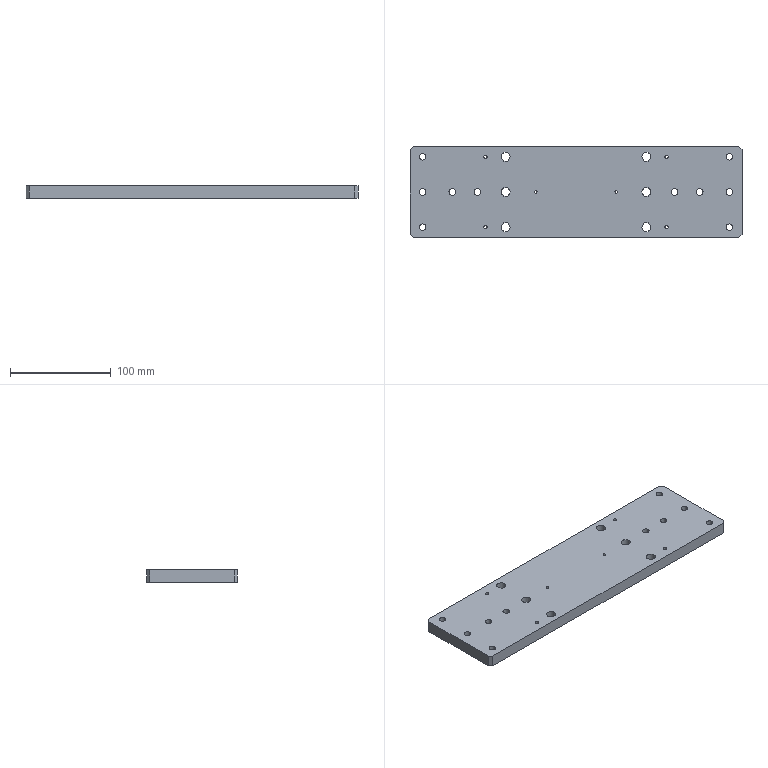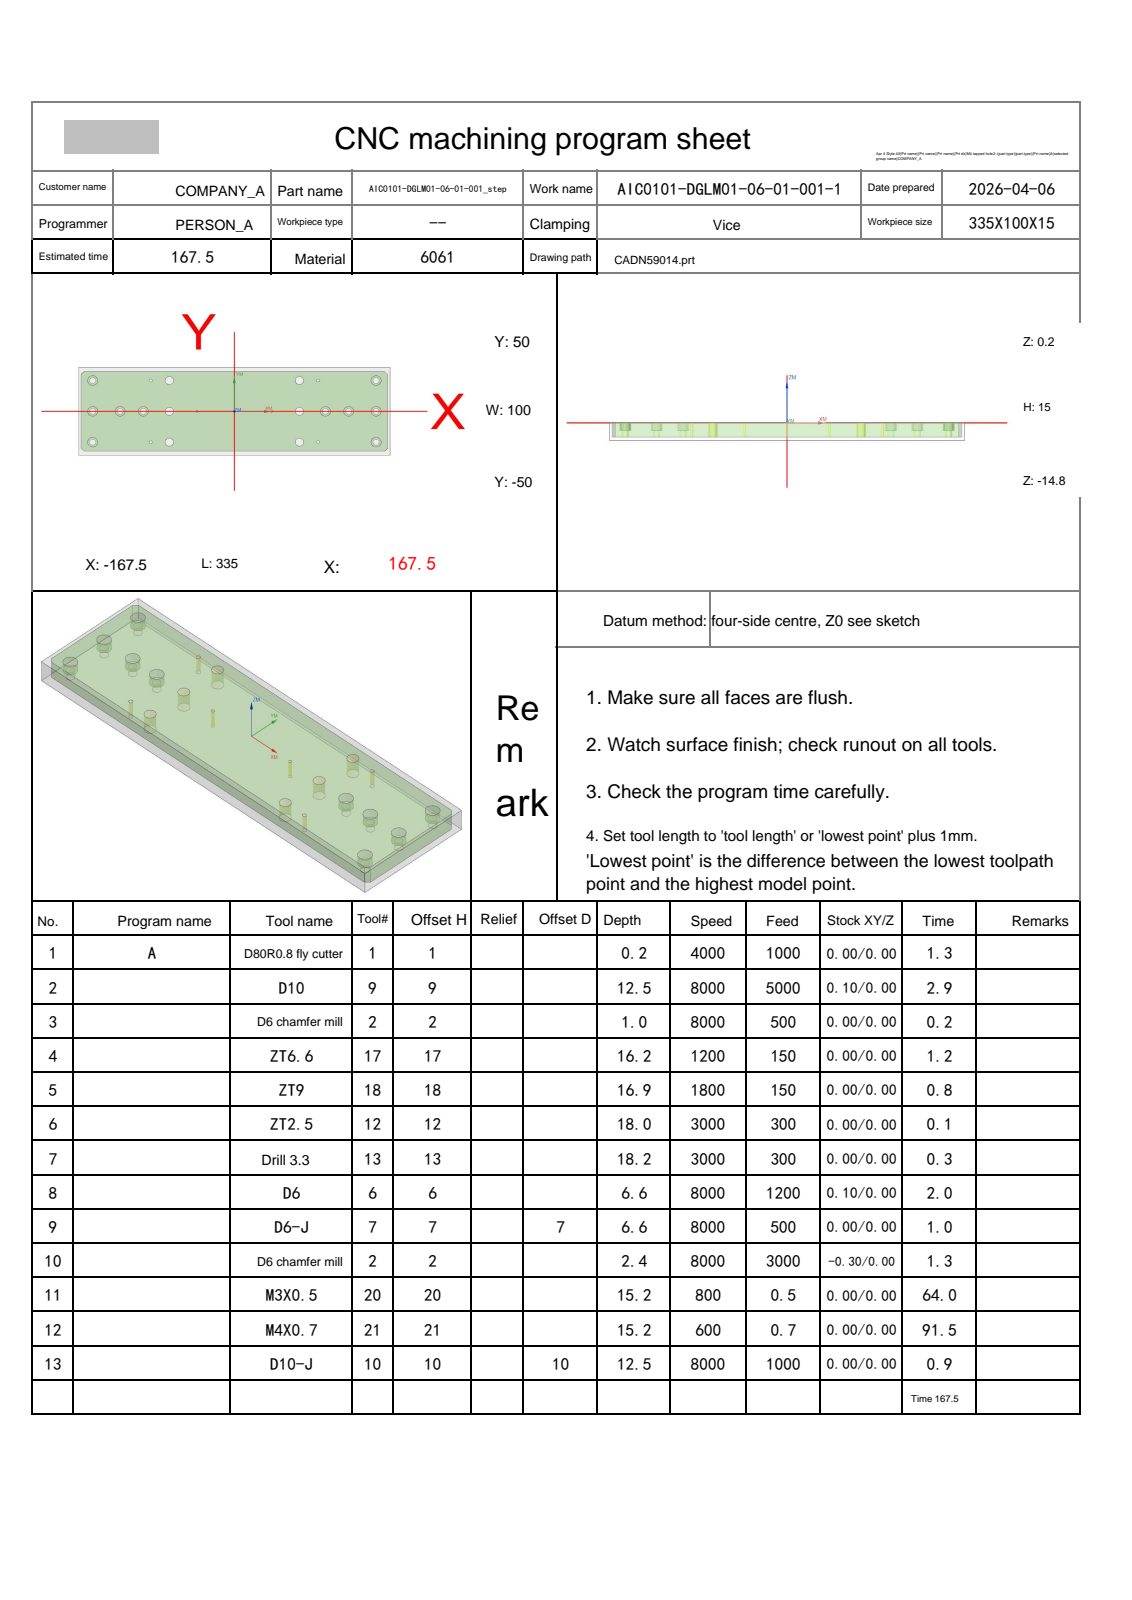NC program | NX | posted by the shop | part box 330 x 90 x 12 mm
Whole program:
%
O0001
(Machine time: 315.72 MIN)
(===Total Tool:12===)
(T1=D80R0.8 fly cutter D=80.  R=0.8  D-  H01 Z=0.    )
(T9=D10     D=10.  R=0.   D-  H09 Z=-12.3 )
(T2=D6 chamfer mill   D=6.   R=0.   D-  H02 Z=-2.2  )
(T17=ZT6.6  D=6.6  DR_a=118 D-  H17 Z=-15.98)
(T18=ZT9    D=9.   DR_a=118 D-  H18 Z=-16.7 )
(T12=ZT2.5  D=2.5  DR_a=118 D-  H12 Z=-17.75)
(T13=drill 3.3  D=3.3  DR_a=118 D-  H13 Z=-17.99)
(T6=D6      D=6.   R=0.   D-  H06 Z=-6.4  )
(T7=D6-J    D=6.   R=0.   D7  H07 Z=-6.4  )
(T20=M3X0.5 D=2.5  DR_a=180 D-  H20 Z=-15.  )
(T21=M4X0.7 D=3.3  DR_a=180 D-  H21 Z=-15.  )
(T10=D10-J  D=10.  R=0.   D10 H10 Z=-12.3 )
G80 G90 G17 G49 G40
G91 G28 Z0
M01
N1 T01 M06
(D80R0.8 fly cutter  D=80. R=0.8 H=01 ce=0.00 di=0.00)
G00 G90 G54 X210. Y-42.5 M03 S4000
G43 H01 Z20.
M08
Z2.
G01 Z0.0 F1000.
X205.
X-205.
Y0.0
X205.
Y42.5
X-205.
X-210.
Z2.
G00 Z20.
G91 G28 Z0.0
M05
M09
G91 G28 Z0.0
M01
N2 T09 M06
(D10  D=10. R=0. H=09 ce=0.10 di=0.00)
G00 G90 G54 X0.0 Y50.1 M03 S8000
G43 H09 Z20.
M08
Z.5
G01 X162. Z.35 F5000.
G02 X165.606 Y48.606 Z.346 I0.0 J-5.1
G01 X168.606 Y45.606 Z.343
G02 X170.1 Y42. Z.339 I-3.606 J-3.606
G01 Y-42. Z.261
G02 X168.606 Y-45.606 Z.257 I-5.1 J0.0
G01 X165.606 Y-48.606 Z.254
G02 X162. Y-50.1 Z.25 I-3.606 J3.606
G01 X-162. Z-.05
G02 X-165.606 Y-48.606 Z-.054 I0.0 J5.1
G01 X-168.606 Y-45.606 Z-.057
G02 X-170.1 Y-42. Z-.061 I3.606 J3.606
G01 Y42. Z-.139
G02 X-168.606 Y45.606 Z-.143 I5.1 J0.0
G01 X-165.606 Y48.606 Z-.146
G02 X-162. Y50.1 Z-.15 I3.606 J-3.606
G01 X162. Z-.45
G02 X165.606 Y48.606 Z-.454 I0.0 J-5.1
G01 X168.606 Y45.606 Z-.457
G02 X170.1 Y42. Z-.461 I-3.606 J-3.606
G01 Y-42. Z-.539
G02 X168.606 Y-45.606 Z-.543 I-5.1 J0.0
G01 X165.606 Y-48.606 Z-.546
G02 X162. Y-50.1 Z-.55 I-3.606 J3.606
G01 X-162. Z-.85
G02 X-165.606 Y-48.606 Z-.854 I0.0 J5.1
G01 X-168.606 Y-45.606 Z-.857
G02 X-170.1 Y-42. Z-.861 I3.606 J3.606
G01 Y42. Z-.939
G02 X-168.606 Y45.606 Z-.943 I5.1 J0.0
G01 X-165.606 Y48.606 Z-.946
G02 X-162. Y50.1 Z-.95 I3.606 J-3.606
G01 X162. Z-1.25
G02 X165.606 Y48.606 Z-1.254 I0.0 J-5.1
G01 X168.606 Y45.606 Z-1.257
G02 X170.1 Y42. Z-1.261 I-3.606 J-3.606
G01 Y-42. Z-1.339
G02 X168.606 Y-45.606 Z-1.343 I-5.1 J0.0
G01 X165.606 Y-48.606 Z-1.346
G02 X162. Y-50.1 Z-1.35 I-3.606 J3.606
G01 X-162. Z-1.65
G02 X-165.606 Y-48.606 Z-1.654 I0.0 J5.1
G01 X-168.606 Y-45.606 Z-1.657
G02 X-170.1 Y-42. Z-1.661 I3.606 J3.606
G01 Y42. Z-1.739
G02 X-168.606 Y45.606 Z-1.743 I5.1 J0.0
G01 X-165.606 Y48.606 Z-1.746
G02 X-162. Y50.1 Z-1.75 I3.606 J-3.606
G01 X162. Z-2.05
G02 X165.606 Y48.606 Z-2.054 I0.0 J-5.1
G01 X168.606 Y45.606 Z-2.057
G02 X170.1 Y42. Z-2.061 I-3.606 J-3.606
G01 Y-42. Z-2.139
G02 X168.606 Y-45.606 Z-2.143 I-5.1 J0.0
G01 X165.606 Y-48.606 Z-2.146
G02 X162. Y-50.1 Z-2.15 I-3.606 J3.606
G01 X-162. Z-2.45
G02 X-165.606 Y-48.606 Z-2.454 I0.0 J5.1
G01 X-168.606 Y-45.606 Z-2.457
G02 X-170.1 Y-42. Z-2.461 I3.606 J3.606
G01 Y42. Z-2.539
G02 X-168.606 Y45.606 Z-2.543 I5.1 J0.0
G01 X-165.606 Y48.606 Z-2.546
G02 X-162. Y50.1 Z-2.55 I3.606 J-3.606
G01 X162. Z-2.85
G02 X165.606 Y48.606 Z-2.854 I0.0 J-5.1
G01 X168.606 Y45.606 Z-2.857
G02 X170.1 Y42. Z-2.861 I-3.606 J-3.606
G01 Y-42. Z-2.939
G02 X168.606 Y-45.606 Z-2.943 I-5.1 J0.0
G01 X165.606 Y-48.606 Z-2.946
G02 X162. Y-50.1 Z-2.95 I-3.606 J3.606
G01 X-162. Z-3.25
G02 X-165.606 Y-48.606 Z-3.254 I0.0 J5.1
G01 X-168.606 Y-45.606 Z-3.257
G02 X-170.1 Y-42. Z-3.261 I3.606 J3.606
G01 Y42. Z-3.339
G02 X-168.606 Y45.606 Z-3.343 I5.1 J0.0
G01 X-165.606 Y48.606 Z-3.346
G02 X-162. Y50.1 Z-3.35 I3.606 J-3.606
G01 X162. Z-3.65
G02 X165.606 Y48.606 Z-3.654 I0.0 J-5.1
G01 X168.606 Y45.606 Z-3.657
G02 X170.1 Y42. Z-3.661 I-3.606 J-3.606
G01 Y-42. Z-3.739
G02 X168.606 Y-45.606 Z-3.743 I-5.1 J0.0
G01 X165.606 Y-48.606 Z-3.746
G02 X162. Y-50.1 Z-3.75 I-3.606 J3.606
G01 X-162. Z-4.05
G02 X-165.606 Y-48.606 Z-4.054 I0.0 J5.1
G01 X-168.606 Y-45.606 Z-4.057
G02 X-170.1 Y-42. Z-4.061 I3.606 J3.606
G01 Y42. Z-4.139
G02 X-168.606 Y45.606 Z-4.143 I5.1 J0.0
G01 X-165.606 Y48.606 Z-4.146
G02 X-162. Y50.1 Z-4.15 I3.606 J-3.606
G01 X162. Z-4.45
G02 X165.606 Y48.606 Z-4.454 I0.0 J-5.1
G01 X168.606 Y45.606 Z-4.457
G02 X170.1 Y42. Z-4.461 I-3.606 J-3.606
G01 Y-42. Z-4.539
G02 X168.606 Y-45.606 Z-4.543 I-5.1 J0.0
G01 X165.606 Y-48.606 Z-4.546
G02 X162. Y-50.1 Z-4.55 I-3.606 J3.606
G01 X-162. Z-4.85
G02 X-165.606 Y-48.606 Z-4.854 I0.0 J5.1
G01 X-168.606 Y-45.606 Z-4.857
G02 X-170.1 Y-42. Z-4.861 I3.606 J3.606
G01 Y42. Z-4.939
G02 X-168.606 Y45.606 Z-4.943 I5.1 J0.0
G01 X-165.606 Y48.606 Z-4.946
G02 X-162. Y50.1 Z-4.95 I3.606 J-3.606
G01 X162. Z-5.25
G02 X165.606 Y48.606 Z-5.254 I0.0 J-5.1
G01 X168.606 Y45.606 Z-5.257
G02 X170.1 Y42. Z-5.261 I-3.606 J-3.606
G01 Y-42. Z-5.339
G02 X168.606 Y-45.606 Z-5.343 I-5.1 J0.0
G01 X165.606 Y-48.606 Z-5.346
G02 X162. Y-50.1 Z-5.35 I-3.606 J3.606
G01 X-162. Z-5.65
G02 X-165.606 Y-48.606 Z-5.654 I0.0 J5.1
G01 X-168.606 Y-45.606 Z-5.657
G02 X-170.1 Y-42. Z-5.661 I3.606 J3.606
G01 Y42. Z-5.739
G02 X-168.606 Y45.606 Z-5.743 I5.1 J0.0
G01 X-165.606 Y48.606 Z-5.746
G02 X-162. Y50.1 Z-5.75 I3.606 J-3.606
G01 X162. Z-6.05
G02 X165.606 Y48.606 Z-6.054 I0.0 J-5.1
G01 X168.606 Y45.606 Z-6.057
G02 X170.1 Y42. Z-6.061 I-3.606 J-3.606
G01 Y-42. Z-6.139
G02 X168.606 Y-45.606 Z-6.143 I-5.1 J0.0
G01 X165.606 Y-48.606 Z-6.146
G02 X162. Y-50.1 Z-6.15 I-3.606 J3.606
G01 X-162. Z-6.45
G02 X-165.606 Y-48.606 Z-6.454 I0.0 J5.1
G01 X-168.606 Y-45.606 Z-6.457
G02 X-170.1 Y-42. Z-6.461 I3.606 J3.606
G01 Y42. Z-6.539
G02 X-168.606 Y45.606 Z-6.543 I5.1 J0.0
G01 X-165.606 Y48.606 Z-6.546
G02 X-162. Y50.1 Z-6.55 I3.606 J-3.606
G01 X162. Z-6.85
G02 X165.606 Y48.606 Z-6.854 I0.0 J-5.1
G01 X168.606 Y45.606 Z-6.857
G02 X170.1 Y42. Z-6.861 I-3.606 J-3.606
G01 Y-42. Z-6.939
G02 X168.606 Y-45.606 Z-6.943 I-5.1 J0.0
G01 X165.606 Y-48.606 Z-6.946
G02 X162. Y-50.1 Z-6.95 I-3.606 J3.606
G01 X-162. Z-7.25
G02 X-165.606 Y-48.606 Z-7.254 I0.0 J5.1
G01 X-168.606 Y-45.606 Z-7.257
G02 X-170.1 Y-42. Z-7.261 I3.606 J3.606
G01 Y42. Z-7.339
G02 X-168.606 Y45.606 Z-7.343 I5.1 J0.0
G01 X-165.606 Y48.606 Z-7.346
G02 X-162. Y50.1 Z-7.35 I3.606 J-3.606
G01 X162. Z-7.65
G02 X165.606 Y48.606 Z-7.654 I0.0 J-5.1
G01 X168.606 Y45.606 Z-7.657
G02 X170.1 Y42. Z-7.661 I-3.606 J-3.606
G01 Y-42. Z-7.739
G02 X168.606 Y-45.606 Z-7.743 I-5.1 J0.0
G01 X165.606 Y-48.606 Z-7.746
G02 X162. Y-50.1 Z-7.75 I-3.606 J3.606
G01 X-162. Z-8.05
G02 X-165.606 Y-48.606 Z-8.054 I0.0 J5.1
G01 X-168.606 Y-45.606 Z-8.057
G02 X-170.1 Y-42. Z-8.061 I3.606 J3.606
G01 Y42. Z-8.139
G02 X-168.606 Y45.606 Z-8.143 I5.1 J0.0
G01 X-165.606 Y48.606 Z-8.146
G02 X-162. Y50.1 Z-8.15 I3.606 J-3.606
G01 X162. Z-8.45
G02 X165.606 Y48.606 Z-8.454 I0.0 J-5.1
G01 X168.606 Y45.606 Z-8.457
G02 X170.1 Y42. Z-8.461 I-3.606 J-3.606
G01 Y-42. Z-8.539
G02 X168.606 Y-45.606 Z-8.543 I-5.1 J0.0
G01 X165.606 Y-48.606 Z-8.546
G02 X162. Y-50.1 Z-8.55 I-3.606 J3.606
G01 X-162. Z-8.85
G02 X-165.606 Y-48.606 Z-8.854 I0.0 J5.1
G01 X-168.606 Y-45.606 Z-8.857
G02 X-170.1 Y-42. Z-8.861 I3.606 J3.606
G01 Y42. Z-8.939
G02 X-168.606 Y45.606 Z-8.943 I5.1 J0.0
G01 X-165.606 Y48.606 Z-8.946
G02 X-162. Y50.1 Z-8.95 I3.606 J-3.606
G01 X162. Z-9.25
G02 X165.606 Y48.606 Z-9.254 I0.0 J-5.1
G01 X168.606 Y45.606 Z-9.257
G02 X170.1 Y42. Z-9.261 I-3.606 J-3.606
G01 Y-42. Z-9.339
G02 X168.606 Y-45.606 Z-9.343 I-5.1 J0.0
G01 X165.606 Y-48.606 Z-9.346
G02 X162. Y-50.1 Z-9.35 I-3.606 J3.606
G01 X-162. Z-9.65
G02 X-165.606 Y-48.606 Z-9.654 I0.0 J5.1
G01 X-168.606 Y-45.606 Z-9.657
G02 X-170.1 Y-42. Z-9.661 I3.606 J3.606
G01 Y42. Z-9.739
G02 X-168.606 Y45.606 Z-9.743 I5.1 J0.0
G01 X-165.606 Y48.606 Z-9.746
G02 X-162. Y50.1 Z-9.75 I3.606 J-3.606
G01 X162. Z-10.05
G02 X165.606 Y48.606 Z-10.054 I0.0 J-5.1
G01 X168.606 Y45.606 Z-10.057
G02 X170.1 Y42. Z-10.061 I-3.606 J-3.606
G01 Y-42. Z-10.139
G02 X168.606 Y-45.606 Z-10.143 I-5.1 J0.0
G01 X165.606 Y-48.606 Z-10.146
G02 X162. Y-50.1 Z-10.15 I-3.606 J3.606
G01 X-162. Z-10.45
G02 X-165.606 Y-48.606 Z-10.454 I0.0 J5.1
G01 X-168.606 Y-45.606 Z-10.457
G02 X-170.1 Y-42. Z-10.461 I3.606 J3.606
G01 Y42. Z-10.539
G02 X-168.606 Y45.606 Z-10.543 I5.1 J0.0
G01 X-165.606 Y48.606 Z-10.546
G02 X-162. Y50.1 Z-10.55 I3.606 J-3.606
G01 X162. Z-10.85
G02 X165.606 Y48.606 Z-10.854 I0.0 J-5.1
G01 X168.606 Y45.606 Z-10.857
G02 X170.1 Y42. Z-10.861 I-3.606 J-3.606
G01 Y-42. Z-10.939
G02 X168.606 Y-45.606 Z-10.943 I-5.1 J0.0
G01 X165.606 Y-48.606 Z-10.946
G02 X162. Y-50.1 Z-10.95 I-3.606 J3.606
G01 X-162. Z-11.25
G02 X-165.606 Y-48.606 Z-11.254 I0.0 J5.1
G01 X-168.606 Y-45.606 Z-11.257
G02 X-170.1 Y-42. Z-11.261 I3.606 J3.606
G01 Y42. Z-11.339
G02 X-168.606 Y45.606 Z-11.343 I5.1 J0.0
G01 X-165.606 Y48.606 Z-11.346
G02 X-162. Y50.1 Z-11.35 I3.606 J-3.606
G01 X162. Z-11.65
G02 X165.606 Y48.606 Z-11.654 I0.0 J-5.1
G01 X168.606 Y45.606 Z-11.657
G02 X170.1 Y42. Z-11.661 I-3.606 J-3.606
G01 Y-42. Z-11.739
G02 X168.606 Y-45.606 Z-11.743 I-5.1 J0.0
G01 X165.606 Y-48.606 Z-11.746
G02 X162. Y-50.1 Z-11.75 I-3.606 J3.606
G01 X-162. Z-12.05
G02 X-165.606 Y-48.606 Z-12.054 I0.0 J5.1
G01 X-168.606 Y-45.606 Z-12.057
G02 X-170.1 Y-42. Z-12.061 I3.606 J3.606
G01 Y42. Z-12.139
G02 X-168.606 Y45.606 Z-12.143 I5.1 J0.0
G01 X-165.606 Y48.606 Z-12.146
G02 X-162. Y50.1 Z-12.15 I3.606 J-3.606
G01 X0.0 Z-12.3
X162.
G02 X165.606 Y48.606 I0.0 J-5.1
G01 X168.606 Y45.606
G02 X170.1 Y42. I-3.606 J-3.606
G01 Y-42.
G02 X168.606 Y-45.606 I-5.1 J0.0
G01 X165.606 Y-48.606
G02 X162. Y-50.1 I-3.606 J3.606
G01 X-162.
G02 X-165.606 Y-48.606 I0.0 J5.1
G01 X-168.606 Y-45.606
G02 X-170.1 Y-42. I3.606 J3.606
G01 Y42.
G02 X-168.606 Y45.606 I5.1 J0.0
G01 X-165.606 Y48.606
G02 X-162. Y50.1 I3.606 J-3.606
G01 X0.0
X.5
Z-11.3
G00 Z20.
G91 G28 Z0.0
M05
M09
G91 G28 Z0.0
M01
N3 T02 M06
(D6 chamfer mill  D=6. R=0. H=02 ce=0.00 di=0.00)
G00 G90 G54 X152.5 Y35. M03 S8000
G43 H02 Z20.
M08
G98 G81 X152.5 Y35. Z-.8 R1. F500.
Y0.0
Y-35.
X123. Y0.0
X98.
X90. Y35.
X70.
Y0.0
X90. Y-35.
X70.
X40. Y0.0
X-40.
X-70. Y-35.
X-90.
X-70. Y0.0
Y35.
X-90.
X-98. Y0.0
X-123.
X-152.5 Y-35.
Y0.0
Y35.
G80
G00 Z20.
G91 G28 Z0.0
M05
M09
G91 G28 Z0.0
M01
N4 T17 M06
(ZT6.6 D=6.6 DR_a=118 H=17)
G00 G90 G54 X-152.5 Y35. M03 S1200
G43 H17 Z20.
M08
G98 G83 X-152.5 Y35. Z-15.983 R1. F150. Q2.
Y0.0
Y-35.
X-123. Y0.0
X-98.
X98.
X123.
X152.5 Y-35.
Y0.0
Y35.
G80
G00 Z20.
G91 G28 Z0.0
M05
M09
G91 G28 Z0.0
M01
N5 T18 M06
(ZT9 D=9. DR_a=118 H=18)
G00 G90 G54 X-70. Y35. M03 S1800
G43 H18 Z20.
M08
G98 G83 X-70. Y35. Z-16.704 R1. F150. Q3.
Y0.0
Y-35.
X70.
Y0.0
Y35.
G80
G00 Z20.
G91 G28 Z0.0
M05
M09
G91 G28 Z0.0
M01
N6 T12 M06
(ZT2.5 D=2.5 DR_a=118 H=12)
G00 G90 G54 X40. Y0.0 M03 S3000
G43 H12 Z20.
M08
G98 G83 X40. Y0.0 Z-17.751 R1. F300. Q2.
X-40.
G80
G00 Z20.
G91 G28 Z0.0
M05
M09
G91 G28 Z0.0
M01
N7 T13 M06
(Drill 3.3 D=3.3 DR_a=118 H=13)
G00 G90 G54 X-90. Y-35. M03 S3000
G43 H13 Z20.
M08
G98 G83 X-90. Y-35. Z-17.991 R1. F300. Q2.
Y35.
X90.
Y-35.
G80
G00 Z20.
G91 G28 Z0.0
M05
M09
G91 G28 Z0.0
M01
N8 T06 M06
(D6  D=6. R=0. H=06 ce=0.10 di=0.00)
G00 G90 G54 X-152.5 Y-35. M03 S8000
G43 H06 Z20.
M08
Z.5
G03 X-151.3 Y-36.2 I1.2 J0.0 F1200.
X-150.1 Y-35. I0.0 J1.2
X-150.1 Y-35. Z0.0 I-2.4 J0.0
X-150.1 Y-35. Z-.5 I-2.4 J0.0
X-150.1 Y-35. Z-1. I-2.4 J0.0
X-150.1 Y-35. Z-1.5 I-2.4 J0.0
X-150.1 Y-35. Z-2. I-2.4 J0.0
X-150.1 Y-35. Z-2.5 I-2.4 J0.0
X-150.1 Y-35. Z-3. I-2.4 J0.0
X-150.1 Y-35. Z-3.5 I-2.4 J0.0
X-150.1 Y-35. Z-4. I-2.4 J0.0
X-150.1 Y-35. Z-4.5 I-2.4 J0.0
X-150.1 Y-35. Z-5. I-2.4 J0.0
X-150.1 Y-35. Z-5.5 I-2.4 J0.0
X-150.1 Y-35. Z-6. I-2.4 J0.0
X-151.758 Y-37.283 Z-6.4 I-2.4 J0.0
X-150.1 Y-35. I-.742 J2.283
X-152.5 Y-32.6 I-2.4 J0.0
X-154.9 Y-35. I0.0 J-2.4
X-152.5 Y-37.4 I2.4 J0.0
X-151.758 Y-37.283 I0.0 J2.4
X-150.929 Y-36.141 I-.371 J1.141
X-152.129 Y-34.941 I-1.2 J0.0
X-152.5 Y-35. I0.0 J-1.2
G00 Z20.
Y0.0
Z.5
G03 X-151.3 Y-1.2 I1.2 J0.0
X-150.1 Y0.0 I0.0 J1.2
X-150.1 Y0.0 Z0.0 I-2.4 J0.0
X-150.1 Y0.0 Z-.5 I-2.4 J0.0
X-150.1 Y0.0 Z-1. I-2.4 J0.0
X-150.1 Y0.0 Z-1.5 I-2.4 J0.0
X-150.1 Y0.0 Z-2. I-2.4 J0.0
X-150.1 Y0.0 Z-2.5 I-2.4 J0.0
X-150.1 Y0.0 Z-3. I-2.4 J0.0
X-150.1 Y0.0 Z-3.5 I-2.4 J0.0
X-150.1 Y0.0 Z-4. I-2.4 J0.0
X-150.1 Y0.0 Z-4.5 I-2.4 J0.0
X-150.1 Y0.0 Z-5. I-2.4 J0.0
X-150.1 Y0.0 Z-5.5 I-2.4 J0.0
X-150.1 Y0.0 Z-6. I-2.4 J0.0
X-151.758 Y-2.283 Z-6.4 I-2.4 J0.0
X-150.1 Y0.0 I-.742 J2.283
X-152.5 Y2.4 I-2.4 J0.0
X-154.9 Y0.0 I0.0 J-2.4
X-152.5 Y-2.4 I2.4 J0.0
X-151.758 Y-2.283 I0.0 J2.4
X-150.929 Y-1.141 I-.371 J1.141
X-152.129 Y.059 I-1.2 J0.0
X-152.5 Y0.0 I0.0 J-1.2
G00 Z20.
Y35.
Z.5
G03 X-151.3 Y33.8 I1.2 J0.0
X-150.1 Y35. I0.0 J1.2
X-150.1 Y35. Z0.0 I-2.4 J0.0
X-150.1 Y35. Z-.5 I-2.4 J0.0
X-150.1 Y35. Z-1. I-2.4 J0.0
X-150.1 Y35. Z-1.5 I-2.4 J0.0
X-150.1 Y35. Z-2. I-2.4 J0.0
X-150.1 Y35. Z-2.5 I-2.4 J0.0
X-150.1 Y35. Z-3. I-2.4 J0.0
X-150.1 Y35. Z-3.5 I-2.4 J0.0
X-150.1 Y35. Z-4. I-2.4 J0.0
X-150.1 Y35. Z-4.5 I-2.4 J0.0
X-150.1 Y35. Z-5. I-2.4 J0.0
X-150.1 Y35. Z-5.5 I-2.4 J0.0
X-150.1 Y35. Z-6. I-2.4 J0.0
X-151.758 Y32.717 Z-6.4 I-2.4 J0.0
X-150.1 Y35. I-.742 J2.283
X-152.5 Y37.4 I-2.4 J0.0
X-154.9 Y35. I0.0 J-2.4
X-152.5 Y32.6 I2.4 J0.0
X-151.758 Y32.717 I0.0 J2.4
X-150.929 Y33.859 I-.371 J1.141
X-152.129 Y35.059 I-1.2 J0.0
X-152.5 Y35. I0.0 J-1.2
G00 Z20.
X-123. Y0.0
Z.5
G03 X-121.8 Y-1.2 I1.2 J0.0
X-120.6 Y0.0 I0.0 J1.2
X-120.6 Y0.0 Z0.0 I-2.4 J0.0
X-120.6 Y0.0 Z-.5 I-2.4 J0.0
X-120.6 Y0.0 Z-1. I-2.4 J0.0
X-120.6 Y0.0 Z-1.5 I-2.4 J0.0
X-120.6 Y0.0 Z-2. I-2.4 J0.0
X-120.6 Y0.0 Z-2.5 I-2.4 J0.0
X-120.6 Y0.0 Z-3. I-2.4 J0.0
X-120.6 Y0.0 Z-3.5 I-2.4 J0.0
X-120.6 Y0.0 Z-4. I-2.4 J0.0
X-120.6 Y0.0 Z-4.5 I-2.4 J0.0
X-120.6 Y0.0 Z-5. I-2.4 J0.0
X-120.6 Y0.0 Z-5.5 I-2.4 J0.0
X-120.6 Y0.0 Z-6. I-2.4 J0.0
X-122.258 Y-2.283 Z-6.4 I-2.4 J0.0
X-120.6 Y0.0 I-.742 J2.283
X-123. Y2.4 I-2.4 J0.0
X-125.4 Y0.0 I0.0 J-2.4
X-123. Y-2.4 I2.4 J0.0
X-122.258 Y-2.283 I0.0 J2.4
X-121.429 Y-1.141 I-.371 J1.141
X-122.629 Y.059 I-1.2 J0.0
X-123. Y0.0 I0.0 J-1.2
G00 Z20.
X-98.
Z.5
G03 X-96.8 Y-1.2 I1.2 J0.0
X-95.6 Y0.0 I0.0 J1.2
X-95.6 Y0.0 Z0.0 I-2.4 J0.0
X-95.6 Y0.0 Z-.5 I-2.4 J0.0
X-95.6 Y0.0 Z-1. I-2.4 J0.0
X-95.6 Y0.0 Z-1.5 I-2.4 J0.0
X-95.6 Y0.0 Z-2. I-2.4 J0.0
X-95.6 Y0.0 Z-2.5 I-2.4 J0.0
X-95.6 Y0.0 Z-3. I-2.4 J0.0
X-95.6 Y0.0 Z-3.5 I-2.4 J0.0
X-95.6 Y0.0 Z-4. I-2.4 J0.0
X-95.6 Y0.0 Z-4.5 I-2.4 J0.0
X-95.6 Y0.0 Z-5. I-2.4 J0.0
X-95.6 Y0.0 Z-5.5 I-2.4 J0.0
X-95.6 Y0.0 Z-6. I-2.4 J0.0
X-97.258 Y-2.283 Z-6.4 I-2.4 J0.0
X-95.6 Y0.0 I-.742 J2.283
X-98. Y2.4 I-2.4 J0.0
X-100.4 Y0.0 I0.0 J-2.4
X-98. Y-2.4 I2.4 J0.0
X-97.258 Y-2.283 I0.0 J2.4
X-96.429 Y-1.141 I-.371 J1.141
X-97.629 Y.059 I-1.2 J0.0
X-98. Y0.0 I0.0 J-1.2
G00 Z20.
X98.
Z.5
G03 X99.2 Y-1.2 I1.2 J0.0
X100.4 Y0.0 I0.0 J1.2
X100.4 Y0.0 Z0.0 I-2.4 J0.0
X100.4 Y0.0 Z-.5 I-2.4 J0.0
X100.4 Y0.0 Z-1. I-2.4 J0.0
X100.4 Y0.0 Z-1.5 I-2.4 J0.0
X100.4 Y0.0 Z-2. I-2.4 J0.0
X100.4 Y0.0 Z-2.5 I-2.4 J0.0
X100.4 Y0.0 Z-3. I-2.4 J0.0
X100.4 Y0.0 Z-3.5 I-2.4 J0.0
X100.4 Y0.0 Z-4. I-2.4 J0.0
X100.4 Y0.0 Z-4.5 I-2.4 J0.0
X100.4 Y0.0 Z-5. I-2.4 J0.0
X100.4 Y0.0 Z-5.5 I-2.4 J0.0
X100.4 Y0.0 Z-6. I-2.4 J0.0
X98.742 Y-2.283 Z-6.4 I-2.4 J0.0
X100.4 Y0.0 I-.742 J2.283
X98. Y2.4 I-2.4 J0.0
X95.6 Y0.0 I0.0 J-2.4
X98. Y-2.4 I2.4 J0.0
X98.742 Y-2.283 I0.0 J2.4
X99.571 Y-1.141 I-.371 J1.141
X98.371 Y.059 I-1.2 J0.0
X98. Y0.0 I0.0 J-1.2
G00 Z20.
X123.
Z.5
G03 X124.2 Y-1.2 I1.2 J0.0
X125.4 Y0.0 I0.0 J1.2
X125.4 Y0.0 Z0.0 I-2.4 J0.0
X125.4 Y0.0 Z-.5 I-2.4 J0.0
X125.4 Y0.0 Z-1. I-2.4 J0.0
X125.4 Y0.0 Z-1.5 I-2.4 J0.0
X125.4 Y0.0 Z-2. I-2.4 J0.0
X125.4 Y0.0 Z-2.5 I-2.4 J0.0
X125.4 Y0.0 Z-3. I-2.4 J0.0
X125.4 Y0.0 Z-3.5 I-2.4 J0.0
X125.4 Y0.0 Z-4. I-2.4 J0.0
X125.4 Y0.0 Z-4.5 I-2.4 J0.0
X125.4 Y0.0 Z-5. I-2.4 J0.0
X125.4 Y0.0 Z-5.5 I-2.4 J0.0
X125.4 Y0.0 Z-6. I-2.4 J0.0
X123.742 Y-2.283 Z-6.4 I-2.4 J0.0
X125.4 Y0.0 I-.742 J2.283
X123. Y2.4 I-2.4 J0.0
X120.6 Y0.0 I0.0 J-2.4
X123. Y-2.4 I2.4 J0.0
X123.742 Y-2.283 I0.0 J2.4
X124.571 Y-1.141 I-.371 J1.141
X123.371 Y.059 I-1.2 J0.0
X123. Y0.0 I0.0 J-1.2
G00 Z20.
X152.5 Y-35.
Z.5
G03 X153.7 Y-36.2 I1.2 J0.0
X154.9 Y-35. I0.0 J1.2
X154.9 Y-35. Z0.0 I-2.4 J0.0
X154.9 Y-35. Z-.5 I-2.4 J0.0
X154.9 Y-35. Z-1. I-2.4 J0.0
X154.9 Y-35. Z-1.5 I-2.4 J0.0
X154.9 Y-35. Z-2. I-2.4 J0.0
X154.9 Y-35. Z-2.5 I-2.4 J0.0
X154.9 Y-35. Z-3. I-2.4 J0.0
X154.9 Y-35. Z-3.5 I-2.4 J0.0
X154.9 Y-35. Z-4. I-2.4 J0.0
X154.9 Y-35. Z-4.5 I-2.4 J0.0
X154.9 Y-35. Z-5. I-2.4 J0.0
X154.9 Y-35. Z-5.5 I-2.4 J0.0
X154.9 Y-35. Z-6. I-2.4 J0.0
X153.242 Y-37.283 Z-6.4 I-2.4 J0.0
X154.9 Y-35. I-.742 J2.283
X152.5 Y-32.6 I-2.4 J0.0
X150.1 Y-35. I0.0 J-2.4
X152.5 Y-37.4 I2.4 J0.0
X153.242 Y-37.283 I0.0 J2.4
X154.071 Y-36.141 I-.371 J1.141
X152.871 Y-34.941 I-1.2 J0.0
X152.5 Y-35. I0.0 J-1.2
G00 Z20.
Y0.0
Z.5
G03 X153.7 Y-1.2 I1.2 J0.0
X154.9 Y0.0 I0.0 J1.2
X154.9 Y0.0 Z0.0 I-2.4 J0.0
X154.9 Y0.0 Z-.5 I-2.4 J0.0
X154.9 Y0.0 Z-1. I-2.4 J0.0
X154.9 Y0.0 Z-1.5 I-2.4 J0.0
X154.9 Y0.0 Z-2. I-2.4 J0.0
X154.9 Y0.0 Z-2.5 I-2.4 J0.0
X154.9 Y0.0 Z-3. I-2.4 J0.0
X154.9 Y0.0 Z-3.5 I-2.4 J0.0
X154.9 Y0.0 Z-4. I-2.4 J0.0
X154.9 Y0.0 Z-4.5 I-2.4 J0.0
X154.9 Y0.0 Z-5. I-2.4 J0.0
X154.9 Y0.0 Z-5.5 I-2.4 J0.0
X154.9 Y0.0 Z-6. I-2.4 J0.0
X153.242 Y-2.283 Z-6.4 I-2.4 J0.0
X154.9 Y0.0 I-.742 J2.283
X152.5 Y2.4 I-2.4 J0.0
X150.1 Y0.0 I0.0 J-2.4
X152.5 Y-2.4 I2.4 J0.0
X153.242 Y-2.283 I0.0 J2.4
X154.071 Y-1.141 I-.371 J1.141
X152.871 Y.059 I-1.2 J0.0
X152.5 Y0.0 I0.0 J-1.2
G00 Z20.
Y35.
Z.5
G03 X153.7 Y33.8 I1.2 J0.0
X154.9 Y35. I0.0 J1.2
X154.9 Y35. Z0.0 I-2.4 J0.0
X154.9 Y35. Z-.5 I-2.4 J0.0
X154.9 Y35. Z-1. I-2.4 J0.0
X154.9 Y35. Z-1.5 I-2.4 J0.0
X154.9 Y35. Z-2. I-2.4 J0.0
X154.9 Y35. Z-2.5 I-2.4 J0.0
X154.9 Y35. Z-3. I-2.4 J0.0
X154.9 Y35. Z-3.5 I-2.4 J0.0
X154.9 Y35. Z-4. I-2.4 J0.0
X154.9 Y35. Z-4.5 I-2.4 J0.0
X154.9 Y35. Z-5. I-2.4 J0.0
X154.9 Y35. Z-5.5 I-2.4 J0.0
X154.9 Y35. Z-6. I-2.4 J0.0
X153.242 Y32.717 Z-6.4 I-2.4 J0.0
X154.9 Y35. I-.742 J2.283
X152.5 Y37.4 I-2.4 J0.0
X150.1 Y35. I0.0 J-2.4
X152.5 Y32.6 I2.4 J0.0
X153.242 Y32.717 I0.0 J2.4
X154.071 Y33.859 I-.371 J1.141
X152.871 Y35.059 I-1.2 J0.0
X152.5 Y35. I0.0 J-1.2
G00 Z20.
G91 G28 Z0.0
M05
M09
G91 G28 Z0.0
M01
N9 T07 M06
(D6-J  D=6. R=0. H=07 ce=0.00 di=0.00)
G00 G90 G54 X-152.5 Y-35. M03 S8000
G43 H07 Z20.
M08
Z0.0
G41 D07
G01 X-152.468 Y-35.197 F500.
G03 X-151.242 Y-36.242 I1.226 J.197
X-150. Y-35. I0.0 J1.242
X-150. Y-35. Z-5. I-2.5 J0.0
X-152.968 Y-32.544 Z-6.4 I-2.5 J0.0
X-155. Y-35. I.468 J-2.456
X-152.5 Y-37.5 I2.5 J0.0
X-150. Y-35. I0.0 J2.5
X-152.5 Y-32.5 I-2.5 J0.0
X-152.968 Y-32.544 I0.0 J-2.5
X-153.978 Y-33.764 I.233 J-1.22
X-152.736 Y-35.006 I1.242 J0.0
G01 X-152.7
G40 X-152.5 Y-35.
G00 Z20.
Y0.0
Z0.0
G41 D07
G01 X-152.468 Y-.197
G03 X-151.242 Y-1.242 I1.226 J.197
X-150. Y0.0 I0.0 J1.242
X-150. Y0.0 Z-5. I-2.5 J0.0
X-152.968 Y2.456 Z-6.4 I-2.5 J0.0
X-155. Y0.0 I.468 J-2.456
X-152.5 Y-2.5 I2.5 J0.0
X-150. Y0.0 I0.0 J2.5
X-152.5 Y2.5 I-2.5 J0.0
X-152.968 Y2.456 I0.0 J-2.5
X-153.978 Y1.236 I.233 J-1.22
X-152.736 Y-.006 I1.242 J0.0
G01 X-152.7
G40 X-152.5 Y0.0
G00 Z20.
Y35.
Z0.0
G41 D07
G01 X-152.468 Y34.803
G03 X-151.242 Y33.758 I1.226 J.197
X-150. Y35. I0.0 J1.242
X-150. Y35. Z-5. I-2.5 J0.0
X-152.968 Y37.456 Z-6.4 I-2.5 J0.0
X-155. Y35. I.468 J-2.456
X-152.5 Y32.5 I2.5 J0.0
X-150. Y35. I0.0 J2.5
X-152.5 Y37.5 I-2.5 J0.0
X-152.968 Y37.456 I0.0 J-2.5
X-153.978 Y36.236 I.233 J-1.22
X-152.736 Y34.994 I1.242 J0.0
G01 X-152.7
G40 X-152.5 Y35.
G00 Z20.
X-123. Y0.0
Z0.0
G41 D07
G01 X-122.968 Y-.197
G03 X-121.742 Y-1.242 I1.226 J.197
X-120.5 Y0.0 I0.0 J1.242
X-120.5 Y0.0 Z-5. I-2.5 J0.0
X-123.468 Y2.456 Z-6.4 I-2.5 J0.0
X-125.5 Y0.0 I.468 J-2.456
X-123. Y-2.5 I2.5 J0.0
X-120.5 Y0.0 I0.0 J2.5
X-123. Y2.5 I-2.5 J0.0
X-123.468 Y2.456 I0.0 J-2.5
X-124.478 Y1.236 I.233 J-1.22
X-123.236 Y-.006 I1.242 J0.0
G01 X-123.2
G40 X-123. Y0.0
G00 Z20.
X-98.
Z0.0
G41 D07
G01 X-97.968 Y-.197
G03 X-96.742 Y-1.242 I1.226 J.197
X-95.5 Y0.0 I0.0 J1.242
X-95.5 Y0.0 Z-5. I-2.5 J0.0
X-98.468 Y2.456 Z-6.4 I-2.5 J0.0
X-100.5 Y0.0 I.468 J-2.456
X-98. Y-2.5 I2.5 J0.0
X-95.5 Y0.0 I0.0 J2.5
X-98. Y2.5 I-2.5 J0.0
X-98.468 Y2.456 I0.0 J-2.5
X-99.478 Y1.236 I.233 J-1.22
X-98.236 Y-.006 I1.242 J0.0
G01 X-98.2
G40 X-98. Y0.0
G00 Z20.
X98.
Z0.0
G41 D07
G01 X98.032 Y-.197
G03 X99.258 Y-1.242 I1.226 J.197
X100.5 Y0.0 I0.0 J1.242
X100.5 Y0.0 Z-5. I-2.5 J0.0
X97.532 Y2.456 Z-6.4 I-2.5 J0.0
X95.5 Y0.0 I.468 J-2.456
X98. Y-2.5 I2.5 J0.0
X100.5 Y0.0 I0.0 J2.5
X98. Y2.5 I-2.5 J0.0
X97.532 Y2.456 I0.0 J-2.5
X96.522 Y1.236 I.233 J-1.22
X97.764 Y-.006 I1.242 J0.0
G01 X97.8
G40 X98. Y0.0
G00 Z20.
X123.
Z0.0
G41 D07
G01 X123.032 Y-.197
G03 X124.258 Y-1.242 I1.226 J.197
X125.5 Y0.0 I0.0 J1.242
X125.5 Y0.0 Z-5. I-2.5 J0.0
X122.532 Y2.456 Z-6.4 I-2.5 J0.0
X120.5 Y0.0 I.468 J-2.456
X123. Y-2.5 I2.5 J0.0
X125.5 Y0.0 I0.0 J2.5
X123. Y2.5 I-2.5 J0.0
X122.532 Y2.456 I0.0 J-2.5
X121.522 Y1.236 I.233 J-1.22
X122.764 Y-.006 I1.242 J0.0
G01 X122.8
G40 X123. Y0.0
G00 Z20.
X152.5 Y-35.
Z0.0
G41 D07
G01 X152.532 Y-35.197
G03 X153.758 Y-36.242 I1.226 J.197
X155. Y-35. I0.0 J1.242
X155. Y-35. Z-5. I-2.5 J0.0
X152.032 Y-32.544 Z-6.4 I-2.5 J0.0
X150. Y-35. I.468 J-2.456
X152.5 Y-37.5 I2.5 J0.0
X155. Y-35. I0.0 J2.5
X152.5 Y-32.5 I-2.5 J0.0
X152.032 Y-32.544 I0.0 J-2.5
X151.022 Y-33.764 I.233 J-1.22
X152.264 Y-35.006 I1.242 J0.0
G01 X152.3
G40 X152.5 Y-35.
G00 Z20.
Y0.0
Z0.0
G41 D07
G01 X152.532 Y-.197
G03 X153.758 Y-1.242 I1.226 J.197
X155. Y0.0 I0.0 J1.242
X155. Y0.0 Z-5. I-2.5 J0.0
X152.032 Y2.456 Z-6.4 I-2.5 J0.0
X150. Y0.0 I.468 J-2.456
X152.5 Y-2.5 I2.5 J0.0
X155. Y0.0 I0.0 J2.5
X152.5 Y2.5 I-2.5 J0.0
X152.032 Y2.456 I0.0 J-2.5
X151.022 Y1.236 I.233 J-1.22
X152.264 Y-.006 I1.242 J0.0
G01 X152.3
G40 X152.5 Y0.0
G00 Z20.
Y35.
Z0.0
G41 D07
G01 X152.532 Y34.803
G03 X153.758 Y33.758 I1.226 J.197
X155. Y35. I0.0 J1.242
X155. Y35. Z-5. I-2.5 J0.0
X152.032 Y37.456 Z-6.4 I-2.5 J0.0
X150. Y35. I.468 J-2.456
X152.5 Y32.5 I2.5 J0.0
X155. Y35. I0.0 J2.5
X152.5 Y37.5 I-2.5 J0.0
X152.032 Y37.456 I0.0 J-2.5
X151.022 Y36.236 I.233 J-1.22
X152.264 Y34.994 I1.242 J0.0
G01 X152.3
G40 X152.5 Y35.
G00 Z20.
G91 G28 Z0.0
M05
M09
G91 G28 Z0.0
M01
N10 T02 M06
(D6 chamfer mill  D=6. R=0. H=02 ce=0.00 di=0.00)
G00 G90 G54 X.25 Y-47.128 M03 S8000
G43 H02 Z20.
M08
Z2.099
G01 Z-1.5 F3000.
G03 X.33 Y-46.828 I-.52 J.3
X.03 Y-46.308 I-.6 J0.0
G01 X0.0 Y-46.3
X-162.
X-162.254 Y-46.275
X-162.497 Y-46.201
X-162.722 Y-46.081
X-162.919 Y-45.919
X-165.919 Y-42.919
X-166.081 Y-42.722
X-166.201 Y-42.497
X-166.275 Y-42.254
X-166.3 Y-42.
Y42.
X-166.275 Y42.254
X-166.201 Y42.497
X-166.081 Y42.722
X-165.919 Y42.919
X-162.919 Y45.919
X-162.722 Y46.081
X-162.497 Y46.201
X-162.254 Y46.275
X-162. Y46.3
X162.
X162.254 Y46.275
X162.497 Y46.201
X162.722 Y46.081
X162.919 Y45.919
X165.919 Y42.919
X166.081 Y42.722
X166.201 Y42.497
X166.275 Y42.254
X166.3 Y42.
Y-42.
X166.275 Y-42.254
X166.201 Y-42.497
X166.081 Y-42.722
X165.919 Y-42.919
X162.919 Y-45.919
X162.722 Y-46.081
X162.497 Y-46.201
X162.254 Y-46.275
X162. Y-46.3
X0.0
X-.03 Y-46.308
G03 X-.33 Y-46.828 I.3 J-.52
X-.25 Y-47.128 I.6 J0.0
G01 Z2.099
G00 Z20.
G00 G90 X40. Y0.0 M03 S8000
Z20.
G98 G81 X40. Y0.0 Z-1.75 R3. F500.
X-40.
G80
G00 Z20.
G00 G90 X-90. Y-35. M03 S8000
Z20.
G98 G81 X-90. Y-35. Z-2.2 R3. F500.
Y35.
X90.
Y-35.
G80
G00 Z20.
G00 G90 X-70.721 Y37.705 M03 S8000
Z20.
Z-.5
G01 Z-1. F800.
X-70.8 Y38.
G03 X-73.8 Y35. I0.0 J-3.
X-70. Y31.2 I3.8 J0.0
X-66.2 Y35. I0.0 J3.8
X-70. Y38.8 I-3.8 J0.0
X-73.8 Y35. I0.0 J-3.8
X-70.8 Y32. I3. J0.0
G01 X-70.721 Y32.295
Z-.5
G00 Z20.
Y2.705
Z-.5
G01 Z-1.
X-70.8 Y3.
G03 X-73.8 Y0.0 I0.0 J-3.
X-70. Y-3.8 I3.8 J0.0
X-66.2 Y0.0 I0.0 J3.8
X-70. Y3.8 I-3.8 J0.0
X-73.8 Y0.0 I0.0 J-3.8
X-70.8 Y-3. I3. J0.0
G01 X-70.721 Y-2.705
Z-.5
G00 Z20.
Y-32.295
Z-.5
G01 Z-1.
X-70.8 Y-32.
G03 X-73.8 Y-35. I0.0 J-3.
X-70. Y-38.8 I3.8 J0.0
X-66.2 Y-35. I0.0 J3.8
X-70. Y-31.2 I-3.8 J0.0
X-73.8 Y-35. I0.0 J-3.8
X-70.8 Y-38. I3. J0.0
G01 X-70.721 Y-37.705
Z-.5
G00 Z20.
X69.279 Y-32.295
Z-.5
G01 Z-1.
X69.2 Y-32.
G03 X66.2 Y-35. I0.0 J-3.
X70. Y-38.8 I3.8 J0.0
X73.8 Y-35. I0.0 J3.8
X70. Y-31.2 I-3.8 J0.0
X66.2 Y-35. I0.0 J-3.8
X69.2 Y-38. I3. J0.0
G01 X69.279 Y-37.705
Z-.5
G00 Z20.
Y2.705
Z-.5
G01 Z-1.
X69.2 Y3.
G03 X66.2 Y0.0 I0.0 J-3.
X70. Y-3.8 I3.8 J0.0
X73.8 Y0.0 I0.0 J3.8
X70. Y3.8 I-3.8 J0.0
X66.2 Y0.0 I0.0 J-3.8
X69.2 Y-3. I3. J0.0
G01 X69.279 Y-2.705
Z-.5
G00 Z20.
Y37.705
Z-.5
G01 Z-1.
X69.2 Y38.
G03 X66.2 Y35. I0.0 J-3.
X70. Y31.2 I3.8 J0.0
X73.8 Y35. I0.0 J3.8
X70. Y38.8 I-3.8 J0.0
X66.2 Y35. I0.0 J-3.8
X69.2 Y32. I3. J0.0
G01 X69.279 Y32.295
Z-.5
G00 Z20.
G00 G90 X-150.491 Y39.357 M03 S8000
Z20.
Z2.5
G01 X-150.666 Y39.439 Z2.43 F800.
X-151.101 Y39.595 Z2.261
X-151.55 Y39.708 Z2.093
X-152.007 Y39.778 Z1.925
X-152.469 Y39.803 Z1.756
X-152.931 Y39.784 Z1.588
X-153.39 Y39.72 Z1.419
X-153.84 Y39.612 Z1.251
X-154.277 Y39.462 Z1.083
X-154.698 Y39.27 Z.914
X-155.099 Y39.039 Z.746
X-155.476 Y38.77 Z.577
X-155.825 Y38.466 Z.409
X-156.143 Y38.13 Z.241
X-156.427 Y37.765 Z.072
X-156.675 Y37.375 Z-.096
X-156.884 Y36.962 Z-.265
X-157.052 Y36.531 Z-.433
X-157.179 Y36.086 Z-.601
X-157.261 Y35.631 Z-.77
X-157.3 Y35.17 Z-.938
Y35. Z-1.
G03 X-152.5 Y30.2 I4.8 J0.0
X-147.7 Y35. I0.0 J4.8
X-152.5 Y39.8 I-4.8 J0.0
X-157.3 Y35. I0.0 J-4.8
X-157.274 Y34.501 I4.8 J0.0
G01 Z1.5
G00 Z20.
X-150.491 Y4.357
Z2.5
G01 X-150.666 Y4.439 Z2.43
X-151.101 Y4.595 Z2.261
X-151.55 Y4.708 Z2.093
X-152.007 Y4.778 Z1.925
X-152.469 Y4.803 Z1.756
X-152.931 Y4.784 Z1.588
X-153.39 Y4.72 Z1.419
X-153.84 Y4.612 Z1.251
X-154.277 Y4.462 Z1.083
X-154.698 Y4.27 Z.914
X-155.099 Y4.039 Z.746
X-155.476 Y3.77 Z.577
X-155.825 Y3.466 Z.409
X-156.143 Y3.13 Z.241
X-156.427 Y2.765 Z.072
X-156.675 Y2.375 Z-.096
X-156.884 Y1.962 Z-.265
X-157.052 Y1.531 Z-.433
X-157.179 Y1.086 Z-.601
X-157.261 Y.631 Z-.77
X-157.3 Y.17 Z-.938
Y0.0 Z-1.
G03 X-152.5 Y-4.8 I4.8 J0.0
X-147.7 Y0.0 I0.0 J4.8
X-152.5 Y4.8 I-4.8 J0.0
X-157.3 Y0.0 I0.0 J-4.8
X-157.274 Y-.499 I4.8 J0.0
G01 Z1.5
G00 Z20.
X-150.491 Y-30.643
Z2.5
G01 X-150.666 Y-30.561 Z2.43
X-151.101 Y-30.405 Z2.261
X-151.55 Y-30.292 Z2.093
X-152.007 Y-30.222 Z1.925
X-152.469 Y-30.197 Z1.756
X-152.931 Y-30.216 Z1.588
X-153.39 Y-30.28 Z1.419
X-153.84 Y-30.388 Z1.251
X-154.277 Y-30.538 Z1.083
X-154.698 Y-30.73 Z.914
X-155.099 Y-30.961 Z.746
X-155.476 Y-31.23 Z.577
X-155.825 Y-31.534 Z.409
X-156.143 Y-31.87 Z.241
X-156.427 Y-32.235 Z.072
X-156.675 Y-32.625 Z-.096
X-156.884 Y-33.038 Z-.265
X-157.052 Y-33.469 Z-.433
X-157.179 Y-33.914 Z-.601
X-157.261 Y-34.369 Z-.77
X-157.3 Y-34.83 Z-.938
Y-35. Z-1.
G03 X-152.5 Y-39.8 I4.8 J0.0
X-147.7 Y-35. I0.0 J4.8
X-152.5 Y-30.2 I-4.8 J0.0
X-157.3 Y-35. I0.0 J-4.8
X-157.274 Y-35.499 I4.8 J0.0
G01 Z1.5
G00 Z20.
X-120.991 Y4.357
Z2.5
G01 X-121.166 Y4.439 Z2.43
X-121.601 Y4.595 Z2.261
X-122.05 Y4.708 Z2.093
X-122.507 Y4.778 Z1.925
X-122.969 Y4.803 Z1.756
X-123.431 Y4.784 Z1.588
X-123.89 Y4.72 Z1.419
X-124.34 Y4.612 Z1.251
X-124.777 Y4.462 Z1.083
X-125.198 Y4.27 Z.914
X-125.599 Y4.039 Z.746
X-125.976 Y3.77 Z.577
X-126.325 Y3.466 Z.409
X-126.643 Y3.13 Z.241
X-126.927 Y2.765 Z.072
X-127.175 Y2.375 Z-.096
X-127.384 Y1.962 Z-.265
X-127.552 Y1.531 Z-.433
X-127.679 Y1.086 Z-.601
X-127.761 Y.631 Z-.77
X-127.8 Y.17 Z-.938
Y0.0 Z-1.
G03 X-123. Y-4.8 I4.8 J0.0
X-118.2 Y0.0 I0.0 J4.8
X-123. Y4.8 I-4.8 J0.0
X-127.8 Y0.0 I0.0 J-4.8
X-127.774 Y-.499 I4.8 J0.0
G01 Z1.5
G00 Z20.
X-95.991 Y4.357
Z2.5
G01 X-96.166 Y4.439 Z2.43
X-96.601 Y4.595 Z2.261
X-97.05 Y4.708 Z2.093
X-97.507 Y4.778 Z1.925
X-97.969 Y4.803 Z1.756
X-98.431 Y4.784 Z1.588
X-98.89 Y4.72 Z1.419
X-99.34 Y4.612 Z1.251
X-99.777 Y4.462 Z1.083
X-100.198 Y4.27 Z.914
X-100.599 Y4.039 Z.746
X-100.976 Y3.77 Z.577
X-101.325 Y3.466 Z.409
X-101.643 Y3.13 Z.241
X-101.927 Y2.765 Z.072
X-102.175 Y2.375 Z-.096
X-102.384 Y1.962 Z-.265
X-102.552 Y1.531 Z-.433
X-102.679 Y1.086 Z-.601
X-102.761 Y.631 Z-.77
X-102.8 Y.17 Z-.938
Y0.0 Z-1.
G03 X-98. Y-4.8 I4.8 J0.0
X-93.2 Y0.0 I0.0 J4.8
X-98. Y4.8 I-4.8 J0.0
X-102.8 Y0.0 I0.0 J-4.8
X-102.774 Y-.499 I4.8 J0.0
G01 Z1.5
G00 Z20.
X100.009 Y4.357
Z2.5
G01 X99.834 Y4.439 Z2.43
X99.399 Y4.595 Z2.261
X98.95 Y4.708 Z2.093
X98.493 Y4.778 Z1.925
X98.031 Y4.803 Z1.756
X97.569 Y4.784 Z1.588
X97.11 Y4.72 Z1.419
X96.66 Y4.612 Z1.251
X96.223 Y4.462 Z1.083
X95.802 Y4.27 Z.914
X95.401 Y4.039 Z.746
X95.024 Y3.77 Z.577
X94.675 Y3.466 Z.409
X94.357 Y3.13 Z.241
X94.073 Y2.765 Z.072
X93.825 Y2.375 Z-.096
X93.616 Y1.962 Z-.265
X93.448 Y1.531 Z-.433
X93.321 Y1.086 Z-.601
X93.239 Y.631 Z-.77
X93.2 Y.17 Z-.938
Y0.0 Z-1.
G03 X98. Y-4.8 I4.8 J0.0
X102.8 Y0.0 I0.0 J4.8
X98. Y4.8 I-4.8 J0.0
X93.2 Y0.0 I0.0 J-4.8
X93.226 Y-.499 I4.8 J0.0
G01 Z1.5
G00 Z20.
X125.009 Y4.357
Z2.5
G01 X124.834 Y4.439 Z2.43
X124.399 Y4.595 Z2.261
X123.95 Y4.708 Z2.093
X123.493 Y4.778 Z1.925
X123.031 Y4.803 Z1.756
X122.569 Y4.784 Z1.588
X122.11 Y4.72 Z1.419
X121.66 Y4.612 Z1.251
X121.223 Y4.462 Z1.083
X120.802 Y4.27 Z.914
X120.401 Y4.039 Z.746
X120.024 Y3.77 Z.577
X119.675 Y3.466 Z.409
X119.357 Y3.13 Z.241
X119.073 Y2.765 Z.072
X118.825 Y2.375 Z-.096
X118.616 Y1.962 Z-.265
X118.448 Y1.531 Z-.433
X118.321 Y1.086 Z-.601
X118.239 Y.631 Z-.77
X118.2 Y.17 Z-.938
Y0.0 Z-1.
G03 X123. Y-4.8 I4.8 J0.0
X127.8 Y0.0 I0.0 J4.8
X123. Y4.8 I-4.8 J0.0
X118.2 Y0.0 I0.0 J-4.8
X118.226 Y-.499 I4.8 J0.0
G01 Z1.5
G00 Z20.
X154.509 Y39.357
Z2.5
G01 X154.334 Y39.439 Z2.43
X153.899 Y39.595 Z2.261
X153.45 Y39.708 Z2.093
X152.993 Y39.778 Z1.925
X152.531 Y39.803 Z1.756
X152.069 Y39.784 Z1.588
X151.61 Y39.72 Z1.419
X151.16 Y39.612 Z1.251
X150.723 Y39.462 Z1.083
X150.302 Y39.27 Z.914
X149.901 Y39.039 Z.746
X149.524 Y38.77 Z.577
X149.175 Y38.466 Z.409
X148.857 Y38.13 Z.241
X148.573 Y37.765 Z.072
X148.325 Y37.375 Z-.096
X148.116 Y36.962 Z-.265
X147.948 Y36.531 Z-.433
X147.821 Y36.086 Z-.601
X147.739 Y35.631 Z-.77
X147.7 Y35.17 Z-.938
Y35. Z-1.
G03 X152.5 Y30.2 I4.8 J0.0
X157.3 Y35. I0.0 J4.8
X152.5 Y39.8 I-4.8 J0.0
X147.7 Y35. I0.0 J-4.8
X147.726 Y34.501 I4.8 J0.0
G01 Z1.5
G00 Z20.
X154.509 Y4.357
Z2.5
G01 X154.334 Y4.439 Z2.43
X153.899 Y4.595 Z2.261
X153.45 Y4.708 Z2.093
X152.993 Y4.778 Z1.925
X152.531 Y4.803 Z1.756
X152.069 Y4.784 Z1.588
X151.61 Y4.72 Z1.419
X151.16 Y4.612 Z1.251
X150.723 Y4.462 Z1.083
X150.302 Y4.27 Z.914
X149.901 Y4.039 Z.746
X149.524 Y3.77 Z.577
X149.175 Y3.466 Z.409
X148.857 Y3.13 Z.241
X148.573 Y2.765 Z.072
X148.325 Y2.375 Z-.096
X148.116 Y1.962 Z-.265
X147.948 Y1.531 Z-.433
X147.821 Y1.086 Z-.601
X147.739 Y.631 Z-.77
X147.7 Y.17 Z-.938
Y0.0 Z-1.
G03 X152.5 Y-4.8 I4.8 J0.0
X157.3 Y0.0 I0.0 J4.8
X152.5 Y4.8 I-4.8 J0.0
X147.7 Y0.0 I0.0 J-4.8
X147.726 Y-.499 I4.8 J0.0
G01 Z1.5
G00 Z20.
X154.509 Y-30.643
Z2.5
G01 X154.334 Y-30.561 Z2.43
X153.899 Y-30.405 Z2.261
X153.45 Y-30.292 Z2.093
X152.993 Y-30.222 Z1.925
X152.531 Y-30.197 Z1.756
X152.069 Y-30.216 Z1.588
X151.61 Y-30.28 Z1.419
X151.16 Y-30.388 Z1.251
X150.723 Y-30.538 Z1.083
X150.302 Y-30.73 Z.914
X149.901 Y-30.961 Z.746
X149.524 Y-31.23 Z.577
X149.175 Y-31.534 Z.409
X148.857 Y-31.87 Z.241
X148.573 Y-32.235 Z.072
X148.325 Y-32.625 Z-.096
X148.116 Y-33.038 Z-.265
X147.948 Y-33.469 Z-.433
X147.821 Y-33.914 Z-.601
X147.739 Y-34.369 Z-.77
X147.7 Y-34.83 Z-.938
Y-35. Z-1.
G03 X152.5 Y-39.8 I4.8 J0.0
X157.3 Y-35. I0.0 J4.8
X152.5 Y-30.2 I-4.8 J0.0
X147.7 Y-35. I0.0 J-4.8
X147.726 Y-35.499 I4.8 J0.0
G01 Z1.5
G00 Z20.
G91 G28 Z0.0
M05
M09
G91 G28 Z0.0
M01
N11 T20 M06
(M3X0.5 D=2.5 DR_a=180 H=20)
G00 G90 G54 X40. Y0.0 M03 S800
G43 H20 Z20.
M08
G95
G98 G84 X40. Y0.0 Z-15. R1. F.5 Q5.
X-40.
G80
G94
G00 Z20.
G91 G28 Z0.0
M05
M09
G91 G28 Z0.0
M01
N12 T21 M06
(M4X0.7 D=3.3 DR_a=180 H=21)
G00 G90 G54 X-90. Y-35. M03 S600
G43 H21 Z20.
M08
G95
G98 G84 X-90. Y-35. Z-15. R1. F.7 Q4.
Y35.
X90.
Y-35.
G80
G94
G00 Z20.
G91 G28 Z0.0
M05
M09
G91 G28 Z0.0
M01
N13 T10 M06
(D10-J  D=10. R=0. H=10 ce=0.00 di=0.00)
G00 G90 G54 X163.013 Y-51.116 M03 S8000
G43 H10 Z20.
M08
Z-11.8
G01 Z-12.3 F1000.
G41 D10
X162.997 Y-50.917
G03 X162. Y-50. I-.997 J-.083
G01 X-162.
G02 X-165.536 Y-48.536 I0.0 J5.
G01 X-168.536 Y-45.536
G02 X-170. Y-42. I3.536 J3.536
G01 Y42.
G02 X-168.536 Y45.536 I5. J0.0
G01 X-165.536 Y48.536
G02 X-162. Y50. I3.536 J-3.536
G01 X162.
G02 X165.536 Y48.536 I0.0 J-5.
G01 X168.536 Y45.536
G02 X170. Y42. I-3.536 J-3.536
G01 Y-42.
G02 X168.536 Y-45.536 I-5. J0.0
G01 X165.536 Y-48.536
G02 X162. Y-50. I-3.536 J3.536
G01 X161.5
G03 X160.5 Y-51. I0.0 J-1.
G01 G40 Y-51.2
Z-11.8
G00 Z20.
M05
M09
G91 G28 Z0.0
G91 G28 Y0.0
M30
%